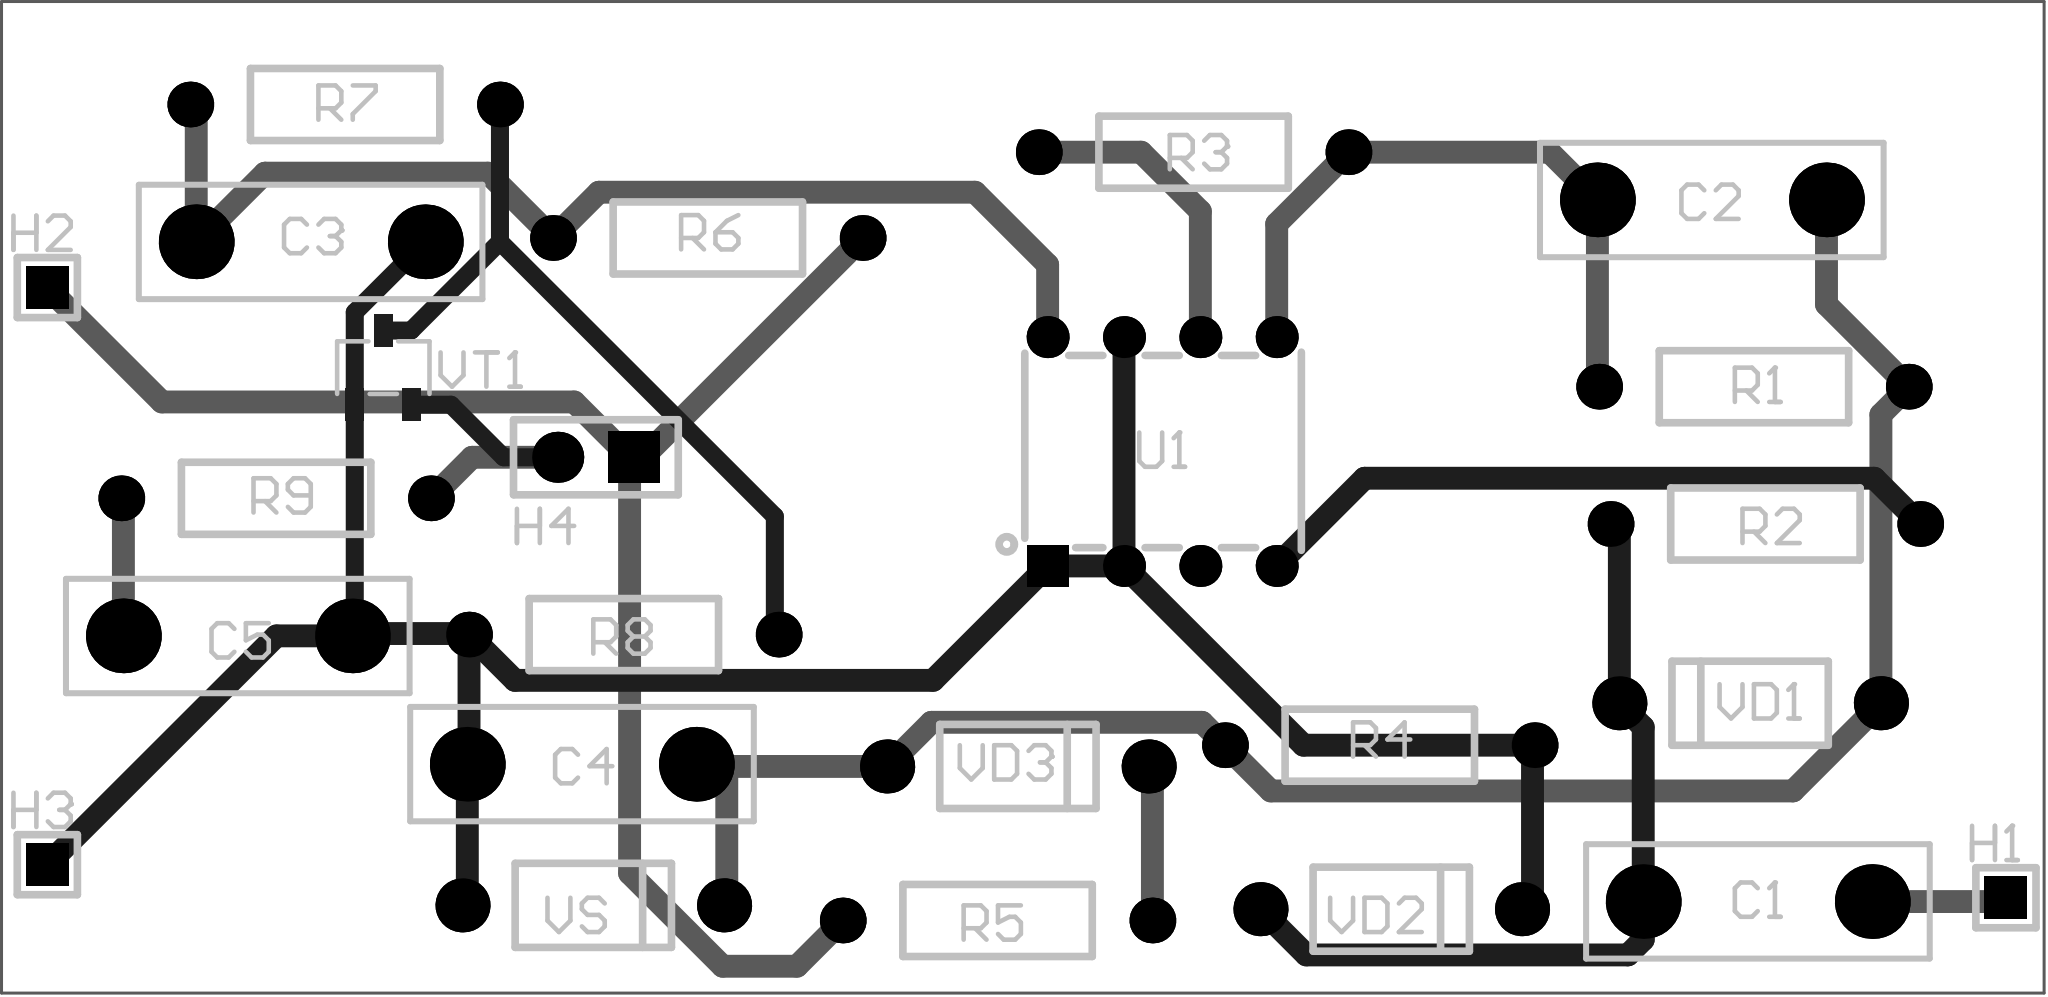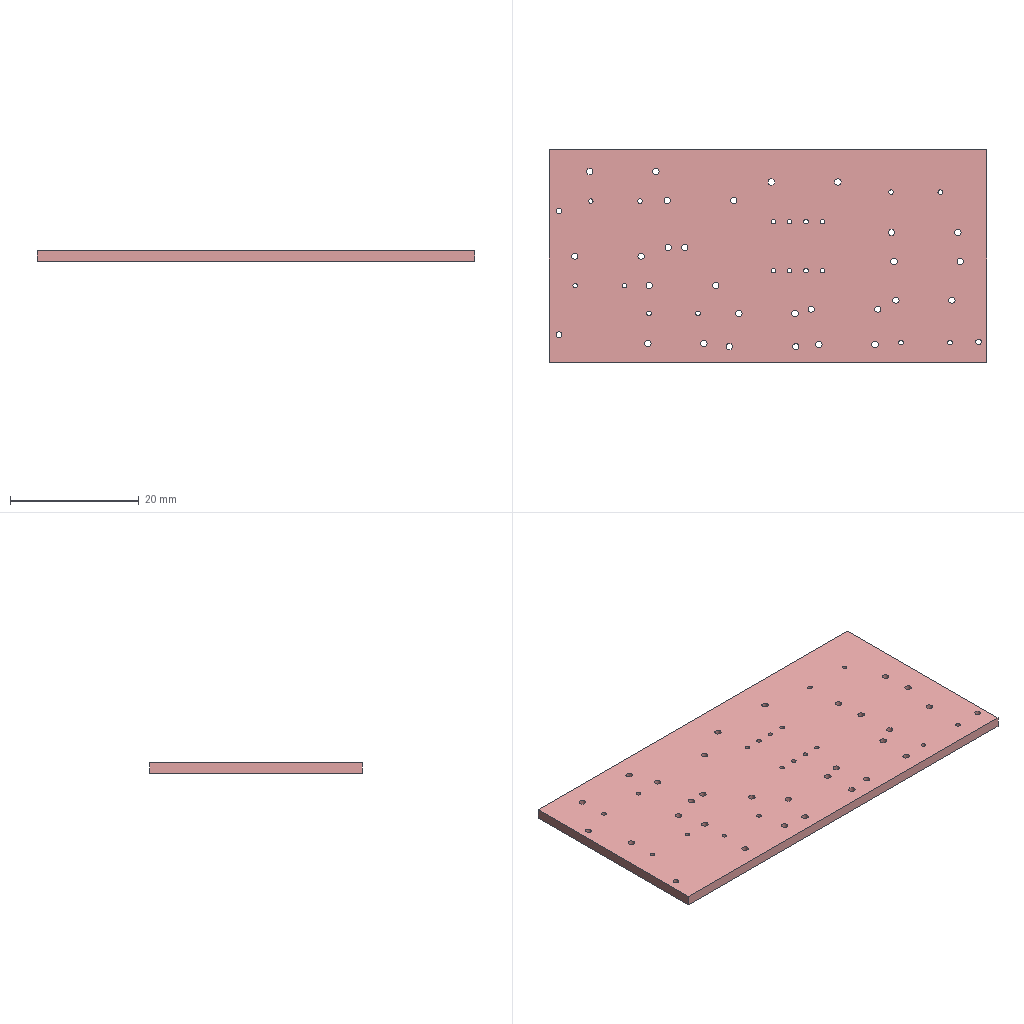Circuit board layout | Altium Designer | box 67.9 x 33 x 1.6 mm
Layer stack:
# Altium Designer layer stack of  (unit mm; dielectric type: 0 none, 1 core, 2 prepreg, 3 surface material)
index,name,kind,layer,copper_thickness_mm,dielectric_type,dielectric_thickness_mm,dielectric_material,dielectric_constant
0,Top Paste Mask Layer,other,,,,,,
1,Top Silkscreen Layer,other,,,,,,
2,Top Solder Mask Layer,dielectric,,,3,0.01,,3.3
3,Top Layer,copper,Top Layer,0.035,,,,
4,Dielectric1,dielectric,,,3,1.51,FR4,4.5
5,Bottom Layer,copper,Bottom Layer,0.035,,,,
6,Bottom Solder Mask Layer,dielectric,,,3,0.01,,3.3
7,Bottom Silkscreen Layer,other,,,,,,
8,Bottom Paste Mask Layer,other,,,,,,
# drill layer pairs: low layer,high layer
drill_pair,Top Layer,Bottom Layer
Part placement:
Designator,Comment,Layer,Footprint,Center-X(mm),Center-Y(mm),Rotation
C1,,TopLayer,RAD-0.3,134.62,79.248,180
C2,,TopLayer,RAD-0.3,133.096,102.616,0
C3,,TopLayer,RAD-0.3,86.487,101.219,0
C4,,TopLayer,RAD-0.3,95.504,83.82,180
C5,,TopLayer,RAD-0.3,84.064,88.096,0
H1,,TopLayer,HDR-TH_1P-V-M_XKB_X4611WV-01I-C28D40,142.875,79.375,0
H2,,TopLayer,HDR-TH_1P-V-M_XKB_X4611WV-01I-C28D40,77.724,99.695,0
H3,,TopLayer,HDR-TH_1P-V-M_XKB_X4611WV-01I-C28D40,77.724,80.475,0
H4,,TopLayer,HDR-TH_2P-P2.54-V-F,95.971,94.043,180
R1,1.5M,TopLayer,Res_1/4W,134.493,96.393,180
R2,1K,TopLayer,Res_1/4W,134.874,91.821,0
R3,20K,TopLayer,Res_1/4W,115.853,104.203,0
R4,360K,TopLayer,Res_1/4W,122.047,84.455,0
R5,39K/2W,TopLayer,Res_1/4W,109.333,78.618,180
R6,2M,TopLayer,Res_1/4W,99.695,101.346,0
R7,100,TopLayer,Res_1/4W,87.63,105.791,0
R8,10K,TopLayer,Res_1/4W,96.901,88.138,0
R9,20,TopLayer,Res_1/4W,85.334,92.677,0
U1,,TopLayer,DIP-8_L9.2-W6.6-P2.54-LS7.62-BL,114.808,94.234,0
VD1,,TopLayer,DO-41_BD2.4-L4.7-P8.70-D0.9-RD,134.366,85.852,0
VD2,1N4148X2,TopLayer,DO-41_BD2.4-L4.7-P8.70-D0.9-RD,122.428,78.994,180
VD3,1N4004,TopLayer,DO-41_BD2.4-L4.7-P8.70-D0.9-RD,110.009,83.747,180
VS,KEL29VI,TopLayer,DO-41_BD2.4-L4.7-P8.70-D0.9-RD,95.885,79.121,180
VT1,97A6,TopLayer,SOT-23-3_L2.9-W1.6-P1.90-LS2.8-BR,88.9,97.028,270
Pad and via stacks:
# Altium Designer via and pad stacks of  (unit mm). Each distinct definition once, with the count of objects using it.
# via: kind,start_layer,end_layer,hole_mm,diameter_mm,mode(0 simple;1 top-mid-bottom;2 full stack),diameter_per_layer,count,example_net
# pad: kind,layer,hole_mm,hole_type(0 round;1 square;2 slot),plating,top_size,top_shape(1 round;2 rect;3 octagon;9 rounded rect),mid_size,bottom_size,mode,footprint,size_per_layer,count,example
pad,Multi-Layer,0.7112,0,plated,2.489x2.489,1,2.489x2.489,2.489x2.489,0,RAD-0.3,,10,C1.2
pad,Multi-Layer,0.9,0,plated,1.4x1.4,2,1.4x1.4,1.4x1.4,0,HDR-TH_1P-V-M_XKB_X4611WV-01I-C28D40,,3,H1.1
pad,Multi-Layer,1,0,plated,1.7x1.7,2,1.7x1.7,1.7x1.7,0,HDR-TH_2P-P2.54-V-F,,1,H4.1
pad,Multi-Layer,1,0,plated,1.7x1.7,1,1.7x1.7,1.7x1.7,0,HDR-TH_2P-P2.54-V-F,,1,H4.2
pad,Multi-Layer,1,0,plated,1.524x1.524,1,1.524x1.524,1.524x1.524,0,Res_1/4W,,18,R1.1
pad,Multi-Layer,0.7112,0,plated,1.397x1.397,1,1.397x1.397,1.397x1.397,0,DIP-8_L9.2-W6.6-P2.54-LS7.62-BL,,7,U1.8
pad,Multi-Layer,0.7112,0,plated,1.397x1.397,2,1.397x1.397,1.397x1.397,0,DIP-8_L9.2-W6.6-P2.54-LS7.62-BL,,1,U1.1
pad,Multi-Layer,1,0,plated,1.8x1.8,1,1.8x1.8,1.8x1.8,0,DO-41_BD2.4-L4.7-P8.70-D0.9-RD,,8,VD1.1
pad,Top Layer,0,0,plated,1.07x0.6,2,1.07x0.6,1.07x0.6,0,SOT-23-3_L2.9-W1.6-P1.90-LS2.8-BR,,3,VT1.1
Design rules, without the lines most boards share:
# Altium Designer design rules of  (exported by Altium Designer, unit mm)
# columns: name | kind | enabled | priority | scope1 | scope2 | descriptor | typed fields (field=value)
copperThickness1oz_2 | 2 | enabled | 2 | All | All | Width Constraint (Min=5mil) (Max=100mil) (Preferred=30mil) (All) |
viaSize | 11 | enabled | 1 | All | All | Routing Via (MinHoleWidth=11.811mil) (MaxHoleWidth=248.032mil) (PreferredHoleWidth=12.008mil) (MinWidth=19.685mil) (MaxWidth=393.701mil) (PreferedWidth=24.016mil) (All) | via_min_hole=0.3 via_max_hole=6.3 via_preferred_diameter=0.61 via_preferred_hole=0.305
solderMaskExpansion | 13 | enabled | 2 | All | All | Solder Mask Expansion (Expansion =2.008mil) (All) | expansion=0.051